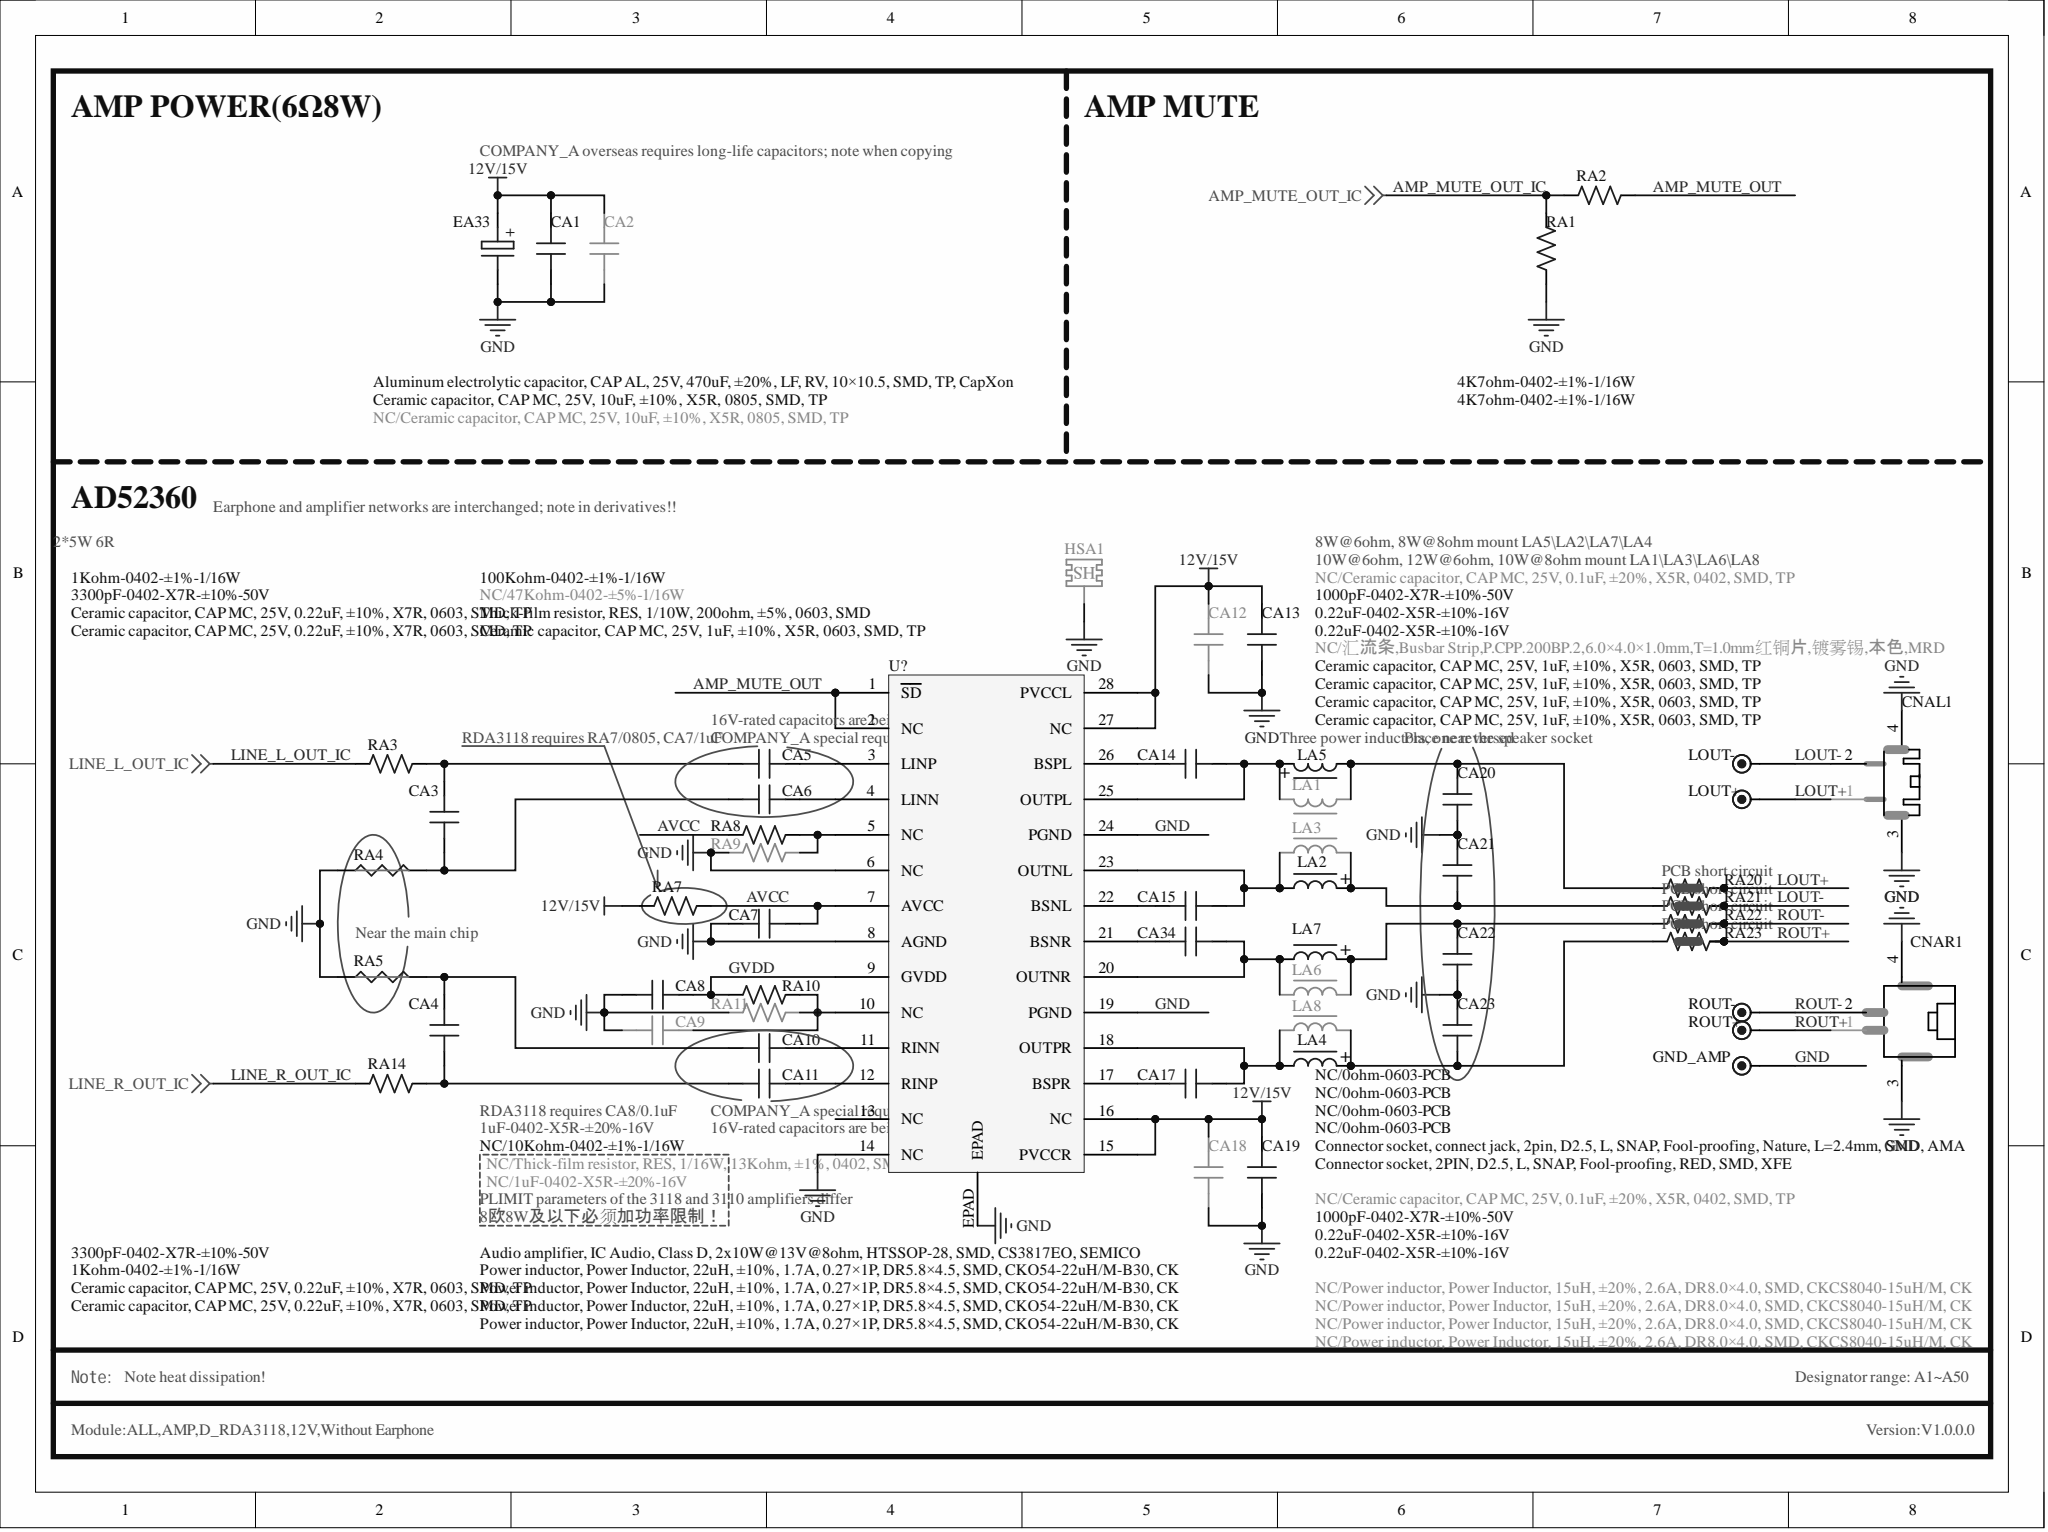Circuit board | Altium Designer | 541 parts | 263 nets | one sheet of the schematic
Parts on this sheet (reference | value | footprint):
CA1 | Ceramic capacitor, CAP MC, 25V, 10uF, ±10%, X5R, 0805, SMD, TP | C0805
CA2 | NC/Ceramic capacitor, CAP MC, 25V, 10uF, ±10%, X5R, 0805, SMD, TP | C0805
CA3 | 3300pF-0402-X7R-±10%-50V | C0402
CA4 | 3300pF-0402-X7R-±10%-50V | C0402
CA5 | Ceramic capacitor, CAP MC, 25V, 0.22uF, ±10%, X7R, 0603, SMD, TP | C0603
CA6 | Ceramic capacitor, CAP MC, 25V, 0.22uF, ±10%, X7R, 0603, SMD, TP | C0603
CA7 | Ceramic capacitor, CAP MC, 25V, 1uF, ±10%, X5R, 0603, SMD, TP | C0603
CA8 | 1uF-0402-X5R-±20%-16V | C0402
CA9 | NC/1uF-0402-X5R-±20%-16V | C0402
CA10 | Ceramic capacitor, CAP MC, 25V, 0.22uF, ±10%, X7R, 0603, SMD, TP | C0603
CA11 | Ceramic capacitor, CAP MC, 25V, 0.22uF, ±10%, X7R, 0603, SMD, TP | C0603
CA12 | NC/Ceramic capacitor, CAP MC, 25V, 0.1uF, ±20%, X5R, 0402, SMD, TP | C0402
CA13 | 1000pF-0402-X7R-±10%-50V | C0402
CA14 | 0.22uF-0402-X5R-±10%-16V | C0402
CA15 | 0.22uF-0402-X5R-±10%-16V | C0402
CA17 | 0.22uF-0402-X5R-±10%-16V | C0402
CA18 | NC/Ceramic capacitor, CAP MC, 25V, 0.1uF, ±20%, X5R, 0402, SMD, TP | C0402
CA19 | 1000pF-0402-X7R-±10%-50V | C0402
CA20 | Ceramic capacitor, CAP MC, 25V, 1uF, ±10%, X5R, 0603, SMD, TP | C0603
CA21 | Ceramic capacitor, CAP MC, 25V, 1uF, ±10%, X5R, 0603, SMD, TP | C0603
CA22 | Ceramic capacitor, CAP MC, 25V, 1uF, ±10%, X5R, 0603, SMD, TP | C0603
CA23 | Ceramic capacitor, CAP MC, 25V, 1uF, ±10%, X5R, 0603, SMD, TP | C0603
CA34 | 0.22uF-0402-X5R-±10%-16V | C0402
CNAL1 | Connector socket, connect jack, 2pin, D2.5, L, SNAP, Fool-proofing, Nature, L=2.4mm, SMD, AMA | SIP2H/2.5S-4
CNAR1 | Connector socket, 2PIN, D2.5, L, SNAP, Fool-proofing, RED, SMD, XFE | SIP2H/2.5S-3
EA33 | Aluminum electrolytic capacitor, CAP AL, 25V, 470uF, ±20%, LF, RV, 10×10.5, SMD, TP, CapXon | EC(10*10.5)-S
GND_AMP | DM0 | TP
HSA1 | NC/汇流条,Busbar Strip,P.CPP.200BP.2,6.0×4.0×1.0mm,T=1.0mm红铜片,镀雾锡,本色,MRD | HL030
LA1 | NC/Power inductor, Power Inductor, 15uH, ±20%, 2.6A, DR8.0×4.0, SMD, CKCS8040-15uH/M, CK | L(8*4.2)-S
LA2 | Power inductor, Power Inductor, 22uH, ±10%, 1.7A, 0.27×1P, DR5.8×4.5, SMD, CKO54-22uH/M-B30, CK | L(5.8*4.5)-S-3
LA3 | NC/Power inductor, Power Inductor, 15uH, ±20%, 2.6A, DR8.0×4.0, SMD, CKCS8040-15uH/M, CK | L(8*4.2)-S
LA4 | Power inductor, Power Inductor, 22uH, ±10%, 1.7A, 0.27×1P, DR5.8×4.5, SMD, CKO54-22uH/M-B30, CK | L(5.8*4.5)-S-3
LA5 | Power inductor, Power Inductor, 22uH, ±10%, 1.7A, 0.27×1P, DR5.8×4.5, SMD, CKO54-22uH/M-B30, CK | L(5.8*4.5)-S-3
LA6 | NC/Power inductor, Power Inductor, 15uH, ±20%, 2.6A, DR8.0×4.0, SMD, CKCS8040-15uH/M, CK | L(8*4.2)-S
LA7 | Power inductor, Power Inductor, 22uH, ±10%, 1.7A, 0.27×1P, DR5.8×4.5, SMD, CKO54-22uH/M-B30, CK | L(5.8*4.5)-S-3
LA8 | NC/Power inductor, Power Inductor, 15uH, ±20%, 2.6A, DR8.0×4.0, SMD, CKCS8040-15uH/M, CK | L(8*4.2)-S
LOUT+ | DM0 | TP
RA1 | 4K7ohm-0402-±1%-1/16W | R0402
RA2 | 4K7ohm-0402-±1%-1/16W | R0402
RA3 | 1Kohm-0402-±1%-1/16W | R0402
RA4 | NC/? | GND
RA5 | NC/? | GND
RA7 | Thick-film resistor, RES, 1/10W, 200ohm, ±5%, 0603, SMD | R0603
RA8 | 100Kohm-0402-±1%-1/16W | R0402
RA9 | NC/47Kohm-0402-±5%-1/16W | R0402
RA10 | NC/10Kohm-0402-±1%-1/16W | R0402
RA11 | NC/Thick-film resistor, RES, 1/16W, 13Kohm, ±1%, 0402, SMD | R0402
RA14 | 1Kohm-0402-±1%-1/16W | R0402
RA20 | NC/0ohm-0603-PCB | R0603SC
RA21 | NC/0ohm-0603-PCB | R0603SC
RA22 | NC/0ohm-0603-PCB | R0603SC
RA23 | NC/0ohm-0603-PCB | R0603SC
ROUT+ | DM0 | TP
U? | Audio amplifier, IC Audio, Class D, 2x10W@13V@8ohm, HTSSOP-28, SMD, CS3817EO, SEMICO | SSOP28/0.65-5
Nets of these parts (net: part-pin ...):
ROUT-: CNAR1-2 RA22-2 RA22-3
ROUT+: CNAR1-1 RA23-2 RA23-3 ROUT+-1
NetRA8_2: RA8-2 RA9-2 U?-5
NetCA34_2: CA34-2 LA6-1 LA7-F U?-20
NetCA34_1: CA34-1 U?-21
NetCA23_1: CA23-1 LA4-S LA8-2 RA23-1
NetCA22_2: CA22-2 LA6-2 LA7-S RA22-1
NetCA21_1: CA21-1 LA2-S LA3-2 RA21-1
NetCA20_2: CA20-2 LA1-1 LA5-F RA20-1
NetCA17_2: CA17-2 LA4-F LA8-1 U?-18
NetCA17_1: CA17-1 U?-17
NetCA15_2: CA15-2 LA2-F LA3-1 U?-23
NetCA15_1: CA15-1 U?-22
NetCA14_2: CA14-2 LA1-2 LA5-S U?-25
NetCA14_1: CA14-1 U?-26
NetCA11_2: CA11-2 U?-12
NetCA10_2: CA10-2 U?-11
NetCA9_2: CA9-2 RA10-2 RA11-2 U?-10
NetCA6_2: CA6-2 U?-4
NetCA5_2: CA5-2 U?-3
NetCA4_2: CA4-2 CA10-1 RA5-JP_1K
NetCA4_1: CA4-1 CA11-1 RA14-2
NetCA3_2: CA3-2 CA5-1 RA3-2
NetCA3_1: CA3-1 CA6-1 RA4-JP_1K
LOUT-: CNAL1-2 RA21-2 RA21-3
LOUT+: CNAL1-1 LOUT+-1 RA20-2 RA20-3
LINE_R_OUT_IC: RA14-1
LINE_L_OUT_IC: RA3-1
GVDD: CA8-2 RA10-1 U?-9
GND: CA1-1 CA2-1 CA7-1 CA8-1 CA9-1 CA12-1 CA13-1 CA18-1 CA19-1 CA20-1 CA21-2 CA22-1 CA23-2 CNAL1-3 CNAL1-4 CNAR1-3 CNAR1-4 EA33-2 GND_AMP-1 HSA1-1 RA1-2 RA4-JP_2K RA5-JP_2K RA9-1 RA11-1 U?-6 U?-8 U?-14 U?-19 U?-24 U?-EPAD
AVCC: CA7-2 RA7-2 RA8-1 U?-7
AMP_MUTE_OUT_IC: RA1-1 RA2-2
AMP_MUTE_OUT: RA2-1 U?-1 U?-2
12V/15V: CA1-2 CA2-2 CA12-2 CA13-2 CA18-2 CA19-2 EA33-1 RA7-1 U?-15 U?-16 U?-27 U?-28